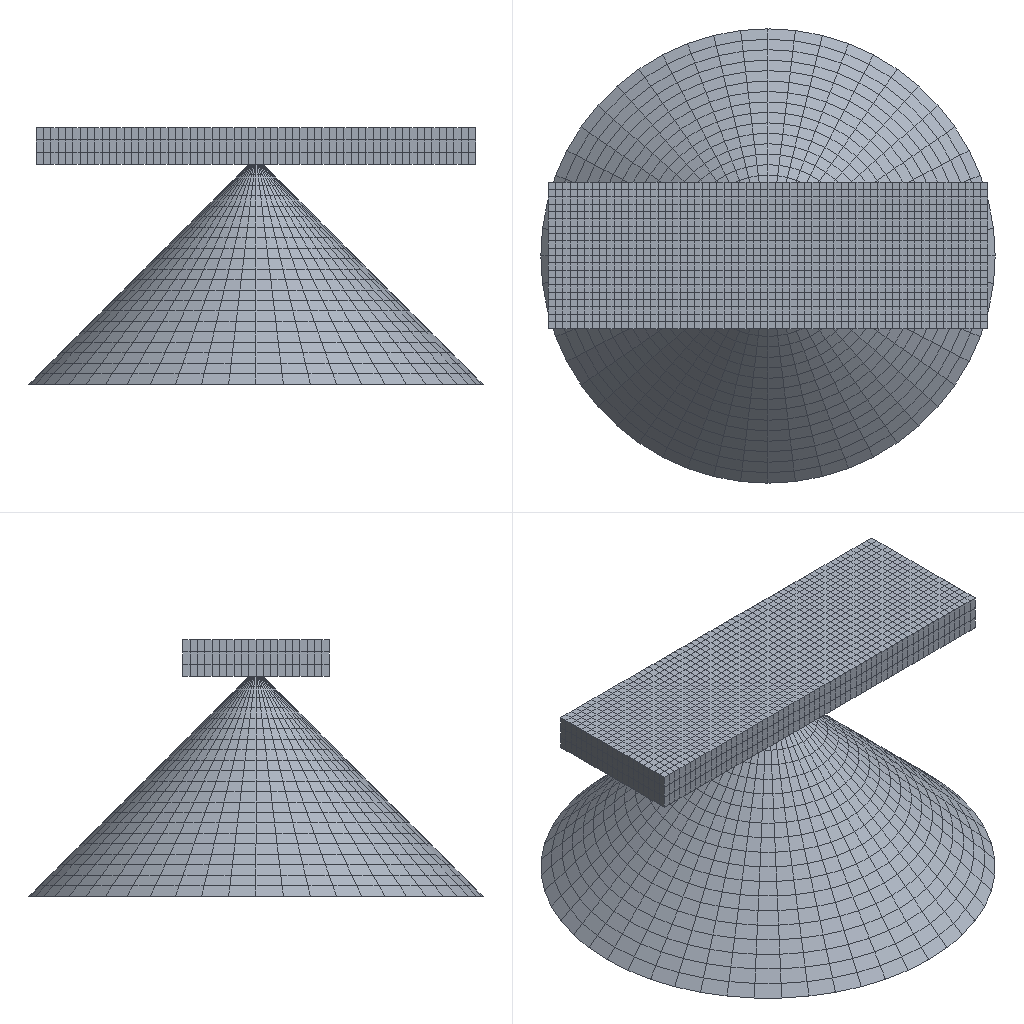Simulation study | abaqus
Set-up summary:
category,name,step,type,value,unit,region
solver,abaqus
solver,version,,,Abaqus/Standard 2020
units,not stated in the deck,,not stated
analysis,deck,,static,static
load_step,Step-1,Step-1,static
load_step,requested,,,1
mesh,nodes,,,9590
mesh,elements,,,7296
element_type,C3D8R,,solid,7296
load,load commands in deck,,count,2
bc,support commands in deck,,count,7
material,JINGANGSHI,,in results
material,YG,,in results
check,setup vs results,,match,"per instance, exact: element labels, types and connectivity; labels of the nodes the elements use; coordinates of those nodes at SINGLE_PRECISION in 1 of 2 instance(s)"
Abaqus input file, long lists of numbers shortened:
*Heading
** Job name: Job-1 Model name: Model-1
** Generated by: Abaqus/CAE 2020
*Preprint, echo=NO, model=NO, history=NO, contact=NO
**
** PARTS
**
*Part, name=ban
*Node
      1,           0.,          -2.,          0.5
      2,           0.,  -1.9,          0.5
** (5122 more lines like these left out)
*Element, type=C3D8R
   1,   85,   86,  107,  106,    1,    2,   23,   22
   2,   86,   87,  108,  107,    2,    3,   24,   23
** (3598 more lines like these left out)
*Nset, nset=Set-4, generate
    1,  5124,     1
*Elset, elset=Set-4, generate
    1,  3600,     1
** Section: yg
*Solid Section, elset=Set-4, material=yg
,
*End Part
**
*Part, name=crack
*End Part
**
*Part, name=jingangshi
*Node
      1, 0.08855,           0., 0.04647
      2, 0.04647,           0., 0.08855
** (4464 more lines like these left out)
*Element, type=C3D8R
   1,   16,   89,   69,   17,  219,  292,  272,  220
   2,   93,   92,   91,  126,  296,  295,  294,  329
** (3694 more lines like these left out)
*Nset, nset=Set-52, generate
    1,  4466,     1
*Elset, elset=Set-52, generate
    1,  3696,     1
*Orientation, name=Ori-1
1., 0., 0., 0., 1., 0.
1, 0.
** Section: jg
*Solid Section, elset=Set-52, orientation=Ori-1, material=jingangshi
,
*End Part
**
**
** ASSEMBLY
**
*Assembly, name=Assembly
**
*Instance, name=ban-1, part=ban
*End Instance
**
*Instance, name=jingangshi-1, part=jingangshi
          3.,          -1.,           0.
          3.,          -1.,           0., 2.,          -1.,           0., 90.
*End Instance
**
*Instance, name=crack-1, part=crack
         3.1,        -0.94,           0.
         3.1,        -0.94,           0.,          3.1, 0.06,           0., 90.
*End Instance
**
*Node
      1,           3.,          -1.,          -3.
*Nset, nset=Set-2
 1,
*Nset, nset=Set-5, instance=ban-1
    1,    2,    3,    4,    5,    6,    7,    8,    9,   10,   11,   12,   13,   14,   15,   16
   17,   18,   19,   20,   21,   85,   86,   87,   88,   89,   90,   91,   92,   93,   94,   95
** (79 more lines like these left out)
*Elset, elset=Set-5, instance=ban-1
    1,    2,    3,    4,    5,    6,    7,    8,    9,   10,   11,   12,   13,   14,   15,   16
   17,   18,   19,   20,   61,   62,   63,   64,   65,   66,   67,   68,   69,   70,   71,   72
** (73 more lines like these left out)
*Nset, nset=Set-6
 1,
*Nset, nset=m_Set-1
 1,
*Nset, nset=_PickedSet12, internal, instance=jingangshi-1, generate
    1,  4466,     1
*Elset, elset=_PickedSet12, internal, instance=jingangshi-1, generate
    1,  3696,     1
*Elset, elset=_m_Surf-2_S1, internal, instance=jingangshi-1, generate
   1,  176,    1
*Surface, type=ELEMENT, name=m_Surf-2
_m_Surf-2_S1, S1
*Elset, elset=_s_Surf-1_S2, internal, instance=jingangshi-1, generate
 3521,  3696,     1
*Surface, type=ELEMENT, name=s_Surf-1
_s_Surf-1_S2, S2
*Elset, elset=_s_Surf-2_S5, internal, instance=ban-1
   41,   42,   43,   44,   45,   46,   47,   48,   49,   50,   51,   52,   53,   54,   55,   56
   57,   58,   59,   60,  101,  102,  103,  104,  105,  106,  107,  108,  109,  110,  111,  112
** (73 more lines like these left out)
*Surface, type=ELEMENT, name=s_Surf-2
_s_Surf-2_S5, S5
** Constraint: Constraint-1
*Coupling, constraint name=Constraint-1, ref node=m_Set-1, surface=s_Surf-1
*Kinematic
*Enrichment, name=Crack-1, type=PROPAGATION CRACK, elset=_PickedSet12
*End Assembly
*Amplitude, name=Amp-1
             0.,              0.,              1.,              1.
**
** MATERIALS
**
*Material, name=jingangshi
*Damage Initiation, criterion=MAXPS
 7e-05,
*Damage Evolution, type=DISPLACEMENT
 1e-07,
*Damage Stabilization
0.001
*Elastic, type=ENGINEERING CONSTANTS
 1.1e+06,900000.,  1e+06,   0.24,    0.2,   0.22,125000.,125000.
125000.,
*Material, name=yg
*Elastic
510000., 0.25
**
** INTERACTION PROPERTIES
**
*Surface Interaction, name=IntProp-1
1.,
*Friction, slip tolerance=0.005
 0.2,
*Surface Behavior, pressure-overclosure=HARD
*Initial Conditions, type=ENRICHMENT
jingangshi-1.8, 1,Crack-1, -0.02316, -0.02293
jingangshi-1.8, 2,Crack-1, -0.03193, -0.01483
jingangshi-1.8, 3,Crack-1, -0.0177, -0.003194
jingangshi-1.8, 4,Crack-1, -0.01145, -0.01353
jingangshi-1.8, 5,Crack-1, 0.08661, 0.03002
jingangshi-1.8, 6,Crack-1, 0.06531, 0.0497
jingangshi-1.8, 7,Crack-1, 0.09987, 0.07796
jingangshi-1.8, 8,Crack-1, 0.115, 0.05286
jingangshi-1.94, 1,Crack-1, -0.04594, -0.02874
jingangshi-1.94, 2,Crack-1, -0.03193, -0.01483
jingangshi-1.94, 3,Crack-1, -0.02316, -0.02293
jingangshi-1.94, 4,Crack-1, -0.03053, -0.03475
jingangshi-1.94, 5,Crack-1, 0.03129, 0.01591
jingangshi-1.94, 6,Crack-1, 0.06531, 0.0497
jingangshi-1.94, 7,Crack-1, 0.08661, 0.03002
jingangshi-1.94, 8,Crack-1, 0.06871, 0.001331
jingangshi-1.56, 1,Crack-1, -0.05402, -0.01638
jingangshi-1.56, 2,Crack-1, -0.0396, -0.005667
jingangshi-1.56, 3,Crack-1, -0.03193, -0.01483
jingangshi-1.56, 4,Crack-1, -0.04594, -0.02874
jingangshi-1.56, 5,Crack-1, 0.01168, 0.04593
jingangshi-1.56, 6,Crack-1, 0.04667, 0.07195
jingangshi-1.56, 7,Crack-1, 0.06531, 0.0497
jingangshi-1.56, 8,Crack-1, 0.03129, 0.01591
jingangshi-1.71, 1,Crack-1, -0.04594, -0.02874
jingangshi-1.71, 2,Crack-1, -0.06393, -0.03983
jingangshi-1.71, 3,Crack-1, -0.06965, -0.02846
jingangshi-1.71, 4,Crack-1, -0.05402, -0.01638
jingangshi-1.71, 5,Crack-1, 0.03129, 0.01591
jingangshi-1.71, 6,Crack-1, -0.0124, 0.001699
jingangshi-1.71, 7,Crack-1, -0.0263, 0.02933
jingangshi-1.71, 8,Crack-1, 0.01168, 0.04593
jingangshi-1.147, 1,Crack-1, -0.04594, -0.02874
jingangshi-1.147, 2,Crack-1, -0.04677, -0.006228
jingangshi-1.147, 3,Crack-1, -0.0594, -0.0906
jingangshi-1.147, 4,Crack-1, -0.06393, -0.03983
jingangshi-1.147, 5,Crack-1, 0.03129, 0.01591
jingangshi-1.147, 6,Crack-1, 0.02928, 0.04286
jingangshi-1.147, 7,Crack-1, -0.001404, 0.04127
jingangshi-1.147, 8,Crack-1, -0.0124, 0.001699
** (104 more lines like these left out)
**
** INTERACTIONS
**
** Interaction: Int-1
*Contact Pair, interaction=IntProp-1, type=SURFACE TO SURFACE
s_Surf-2, m_Surf-2
** ----------------------------------------------------------------
**
** STEP: Step-1
**
*Step, name=Step-1, nlgeom=YES, inc=1000
*Static, stabilize=0.0002, allsdtol=0.05, continue=NO
0.01, 1., 1e-07, 1.
**
** BOUNDARY CONDITIONS
**
** Name: BC-1 Type: 对称/反对称/完全固定
*Boundary
Set-5, ENCASTRE
** Name: [REDACTED] : Displacement/rotation angle
*Boundary, amplitude=Amp-1
Set-6, 1, 1, 0.6
Set-6, 2, 2
Set-6, 3, 3
Set-6, 4, 4
Set-6, 5, 5
Set-6, 6, 6
**
** LOADS
**
** Name: Load-1   Type: Concentrated force
*Cload
Set-2, 3, 120.
**
** INTERACTIONS
**
** Interaction: Int-2
*Enrichment Activation, name=Crack-1, activate=ON
**
** CONTROLS
**
*Controls, reset
*Controls, parameters=time incrementation
, , , , , , , 20, , ,
**
** OUTPUT REQUESTS
**
*Restart, write, frequency=0
**
** FIELD OUTPUT: F-Output-1
**
*Output, field
*Node Output
CF, PHILSM, PSILSM, RF, RM, RT, TF, U
V
*Element Output, directions=YES
E, ENRRTXFEM, LE, MISES, MISESMAX, MISESONLY, PE, PEEQ, PEEQMAX, PEEQT, PEMAG, S, SDEG, SF, SSAVG, STATUS
*Contact Output
CDISP, CSTRESS
*Output, history, frequency=0
*End Step
Results summary:
result,step,,completed,increments=153 time=1.0/1.0
result,analysis,,,static
result,last_loadstep,,,1
result,primary field,,,U
result,reaction total,,FX,-0.0,model units
result,reaction total,,FY,-0.0,model units
result,reaction total,,FZ,-120,model units